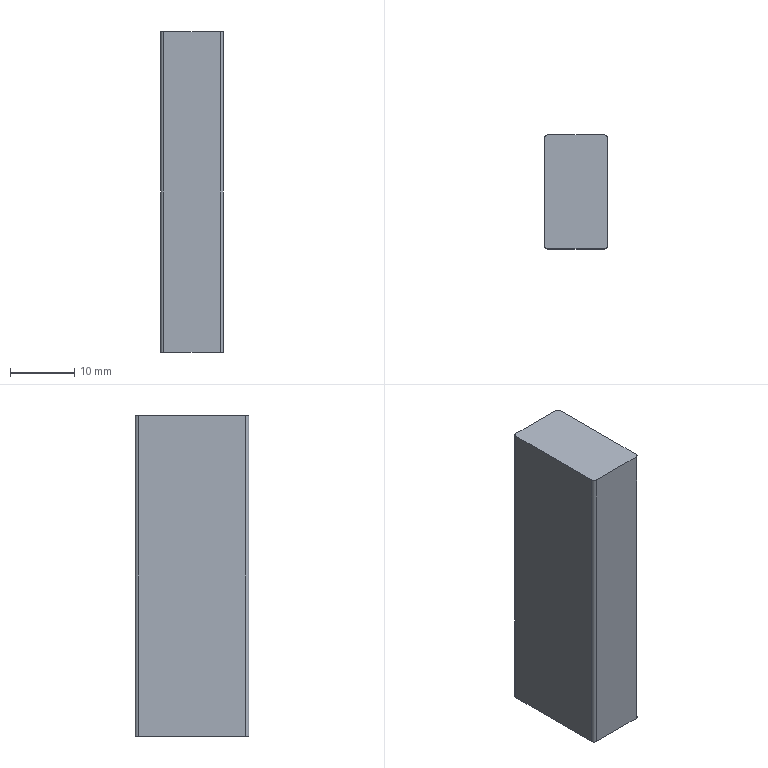Part | NX | features BREP 1 | 1 solid | 10 faces | box 9.8 x 17.754 x 50 mm | volume 8689 mm3 | plane 6 | cylinder 4 | commonest cylinder face diameters 1 x4
STEP:
#1=CARTESIAN_POINT('',(-4.4,8.877,-40.6));
#2=VERTEX_POINT('',#1);
#3=CARTESIAN_POINT('',(-4.9,8.377,-40.6));
#4=VERTEX_POINT('',#3);
#5=CARTESIAN_POINT('',(-4.4,8.377,-40.6));
#6=DIRECTION('',(0.,0.,1.));
#7=DIRECTION('',(1.,0.,0.));
#8=AXIS2_PLACEMENT_3D('',#5,#6,#7);
#9=CIRCLE('',#8,0.5);
#10=EDGE_CURVE('',#2,#4,#9,.T.);
#11=ORIENTED_EDGE('',*,*,#10,.F.);
#12=CARTESIAN_POINT('',(-4.4,8.877,-90.6));
#13=VERTEX_POINT('',#12);
#14=CARTESIAN_POINT('',(-4.4,8.877,-90.6));
#15=DIRECTION('',(0.,0.,1.));
#16=VECTOR('',#15,1000.);
#17=LINE('',#14,#16);
#18=EDGE_CURVE('',#13,#2,#17,.T.);
#19=ORIENTED_EDGE('',*,*,#18,.F.);
#20=CARTESIAN_POINT('',(-4.9,8.377,-90.6));
#21=VERTEX_POINT('',#20);
#22=CARTESIAN_POINT('',(-4.4,8.377,-90.6));
#23=DIRECTION('',(0.,0.,1.));
#24=DIRECTION('',(1.,0.,0.));
#25=AXIS2_PLACEMENT_3D('',#22,#23,#24);
#26=CIRCLE('',#25,0.5);
#27=EDGE_CURVE('',#13,#21,#26,.T.);
#28=ORIENTED_EDGE('',*,*,#27,.T.);
#29=CARTESIAN_POINT('',(-4.9,8.377,-90.6));
#30=DIRECTION('',(0.,0.,1.));
#31=VECTOR('',#30,1000.);
#32=LINE('',#29,#31);
#33=EDGE_CURVE('',#21,#4,#32,.T.);
#34=ORIENTED_EDGE('',*,*,#33,.T.);
#35=EDGE_LOOP('',(#11,#19,#28,#34));
#36=FACE_BOUND('',#35,.T.);
#37=CARTESIAN_POINT('',(-4.4,8.377,-90.6));
#38=DIRECTION('',(0.,0.,1.));
#39=DIRECTION('',(-1.,0.,0.));
#40=AXIS2_PLACEMENT_3D('',#37,#38,#39);
#41=CYLINDRICAL_SURFACE('',#40,0.5);
#42=ADVANCED_FACE('',(#36),#41,.T.);
#43=CARTESIAN_POINT('',(-4.9,-8.377,-40.6));
#44=VERTEX_POINT('',#43);
#45=CARTESIAN_POINT('',(-4.9,-8.377,-40.6));
#46=DIRECTION('',(0.,1.,0.));
#47=VECTOR('',#46,1000.);
#48=LINE('',#45,#47);
#49=EDGE_CURVE('',#44,#4,#48,.T.);
#50=ORIENTED_EDGE('',*,*,#49,.T.);
#51=ORIENTED_EDGE('',*,*,#33,.F.);
#52=CARTESIAN_POINT('',(-4.9,-8.377,-90.6));
#53=VERTEX_POINT('',#52);
#54=CARTESIAN_POINT('',(-4.9,-8.377,-90.6));
#55=DIRECTION('',(0.,1.,0.));
#56=VECTOR('',#55,1000.);
#57=LINE('',#54,#56);
#58=EDGE_CURVE('',#53,#21,#57,.T.);
#59=ORIENTED_EDGE('',*,*,#58,.F.);
#60=CARTESIAN_POINT('',(-4.9,-8.377,-90.6));
#61=DIRECTION('',(0.,0.,1.));
#62=VECTOR('',#61,1000.);
#63=LINE('',#60,#62);
#64=EDGE_CURVE('',#53,#44,#63,.T.);
#65=ORIENTED_EDGE('',*,*,#64,.T.);
#66=EDGE_LOOP('',(#50,#51,#59,#65));
#67=FACE_BOUND('',#66,.T.);
#68=CARTESIAN_POINT('',(-4.9,-8.377,-90.6));
#69=DIRECTION('',(1.,0.,0.));
#70=DIRECTION('',(0.,-1.,0.));
#71=AXIS2_PLACEMENT_3D('',#68,#69,#70);
#72=PLANE('',#71);
#73=ADVANCED_FACE('',(#67),#72,.F.);
#74=CARTESIAN_POINT('',(-4.4,-8.877,-40.6));
#75=VERTEX_POINT('',#74);
#76=CARTESIAN_POINT('',(-4.4,-8.377,-40.6));
#77=DIRECTION('',(0.,0.,1.));
#78=DIRECTION('',(1.,0.,0.));
#79=AXIS2_PLACEMENT_3D('',#76,#77,#78);
#80=CIRCLE('',#79,0.5);
#81=EDGE_CURVE('',#44,#75,#80,.T.);
#82=ORIENTED_EDGE('',*,*,#81,.F.);
#83=ORIENTED_EDGE('',*,*,#64,.F.);
#84=CARTESIAN_POINT('',(-4.4,-8.877,-90.6));
#85=VERTEX_POINT('',#84);
#86=CARTESIAN_POINT('',(-4.4,-8.377,-90.6));
#87=DIRECTION('',(0.,0.,1.));
#88=DIRECTION('',(1.,0.,0.));
#89=AXIS2_PLACEMENT_3D('',#86,#87,#88);
#90=CIRCLE('',#89,0.5);
#91=EDGE_CURVE('',#53,#85,#90,.T.);
#92=ORIENTED_EDGE('',*,*,#91,.T.);
#93=CARTESIAN_POINT('',(-4.4,-8.877,-90.6));
#94=DIRECTION('',(0.,0.,1.));
#95=VECTOR('',#94,1000.);
#96=LINE('',#93,#95);
#97=EDGE_CURVE('',#85,#75,#96,.T.);
#98=ORIENTED_EDGE('',*,*,#97,.T.);
#99=EDGE_LOOP('',(#82,#83,#92,#98));
#100=FACE_BOUND('',#99,.T.);
#101=CARTESIAN_POINT('',(-4.4,-8.377,-90.6));
#102=DIRECTION('',(0.,0.,1.));
#103=DIRECTION('',(-1.,0.,0.));
#104=AXIS2_PLACEMENT_3D('',#101,#102,#103);
#105=CYLINDRICAL_SURFACE('',#104,0.5);
#106=ADVANCED_FACE('',(#100),#105,.T.);
#107=CARTESIAN_POINT('',(4.4,-8.877,-40.6));
#108=VERTEX_POINT('',#107);
#109=CARTESIAN_POINT('',(4.4,-8.877,-40.6));
#110=DIRECTION('',(-1.,0.,0.));
#111=VECTOR('',#110,1000.);
#112=LINE('',#109,#111);
#113=EDGE_CURVE('',#108,#75,#112,.T.);
#114=ORIENTED_EDGE('',*,*,#113,.T.);
#115=ORIENTED_EDGE('',*,*,#97,.F.);
#116=CARTESIAN_POINT('',(4.4,-8.877,-90.6));
#117=VERTEX_POINT('',#116);
#118=CARTESIAN_POINT('',(4.4,-8.877,-90.6));
#119=DIRECTION('',(-1.,0.,0.));
#120=VECTOR('',#119,1000.);
#121=LINE('',#118,#120);
#122=EDGE_CURVE('',#117,#85,#121,.T.);
#123=ORIENTED_EDGE('',*,*,#122,.F.);
#124=CARTESIAN_POINT('',(4.4,-8.877,-90.6));
#125=DIRECTION('',(0.,0.,1.));
#126=VECTOR('',#125,1000.);
#127=LINE('',#124,#126);
#128=EDGE_CURVE('',#117,#108,#127,.T.);
#129=ORIENTED_EDGE('',*,*,#128,.T.);
#130=EDGE_LOOP('',(#114,#115,#123,#129));
#131=FACE_BOUND('',#130,.T.);
#132=CARTESIAN_POINT('',(4.4,-8.877,-90.6));
#133=DIRECTION('',(0.,1.,0.));
#134=DIRECTION('',(0.,0.,-1.));
#135=AXIS2_PLACEMENT_3D('',#132,#133,#134);
#136=PLANE('',#135);
#137=ADVANCED_FACE('',(#131),#136,.F.);
#138=CARTESIAN_POINT('',(4.9,-8.377,-40.6));
#139=VERTEX_POINT('',#138);
#140=CARTESIAN_POINT('',(4.4,-8.377,-40.6));
#141=DIRECTION('',(0.,0.,1.));
#142=DIRECTION('',(1.,0.,0.));
#143=AXIS2_PLACEMENT_3D('',#140,#141,#142);
#144=CIRCLE('',#143,0.5);
#145=EDGE_CURVE('',#108,#139,#144,.T.);
#146=ORIENTED_EDGE('',*,*,#145,.F.);
#147=ORIENTED_EDGE('',*,*,#128,.F.);
#148=CARTESIAN_POINT('',(4.9,-8.377,-90.6));
#149=VERTEX_POINT('',#148);
#150=CARTESIAN_POINT('',(4.4,-8.377,-90.6));
#151=DIRECTION('',(0.,0.,1.));
#152=DIRECTION('',(1.,0.,0.));
#153=AXIS2_PLACEMENT_3D('',#150,#151,#152);
#154=CIRCLE('',#153,0.5);
#155=EDGE_CURVE('',#117,#149,#154,.T.);
#156=ORIENTED_EDGE('',*,*,#155,.T.);
#157=CARTESIAN_POINT('',(4.9,-8.377,-90.6));
#158=DIRECTION('',(0.,0.,1.));
#159=VECTOR('',#158,1000.);
#160=LINE('',#157,#159);
#161=EDGE_CURVE('',#149,#139,#160,.T.);
#162=ORIENTED_EDGE('',*,*,#161,.T.);
#163=EDGE_LOOP('',(#146,#147,#156,#162));
#164=FACE_BOUND('',#163,.T.);
#165=CARTESIAN_POINT('',(4.4,-8.377,-90.6));
#166=DIRECTION('',(0.,0.,1.));
#167=DIRECTION('',(-1.,0.,0.));
#168=AXIS2_PLACEMENT_3D('',#165,#166,#167);
#169=CYLINDRICAL_SURFACE('',#168,0.5);
#170=ADVANCED_FACE('',(#164),#169,.T.);
#171=CARTESIAN_POINT('',(4.9,8.377,-40.6));
#172=VERTEX_POINT('',#171);
#173=CARTESIAN_POINT('',(4.9,8.377,-40.6));
#174=DIRECTION('',(0.,-1.,0.));
#175=VECTOR('',#174,1000.);
#176=LINE('',#173,#175);
#177=EDGE_CURVE('',#172,#139,#176,.T.);
#178=ORIENTED_EDGE('',*,*,#177,.T.);
#179=ORIENTED_EDGE('',*,*,#161,.F.);
#180=CARTESIAN_POINT('',(4.9,8.377,-90.6));
#181=VERTEX_POINT('',#180);
#182=CARTESIAN_POINT('',(4.9,8.377,-90.6));
#183=DIRECTION('',(0.,-1.,0.));
#184=VECTOR('',#183,1000.);
#185=LINE('',#182,#184);
#186=EDGE_CURVE('',#181,#149,#185,.T.);
#187=ORIENTED_EDGE('',*,*,#186,.F.);
#188=CARTESIAN_POINT('',(4.9,8.377,-90.6));
#189=DIRECTION('',(0.,0.,1.));
#190=VECTOR('',#189,1000.);
#191=LINE('',#188,#190);
#192=EDGE_CURVE('',#181,#172,#191,.T.);
#193=ORIENTED_EDGE('',*,*,#192,.T.);
#194=EDGE_LOOP('',(#178,#179,#187,#193));
#195=FACE_BOUND('',#194,.T.);
#196=CARTESIAN_POINT('',(4.9,8.377,-90.6));
#197=DIRECTION('',(-1.,0.,0.));
#198=DIRECTION('',(0.,0.,-1.));
#199=AXIS2_PLACEMENT_3D('',#196,#197,#198);
#200=PLANE('',#199);
#201=ADVANCED_FACE('',(#195),#200,.F.);
#202=CARTESIAN_POINT('',(4.4,8.877,-40.6));
#203=VERTEX_POINT('',#202);
#204=CARTESIAN_POINT('',(4.4,8.377,-40.6));
#205=DIRECTION('',(0.,0.,1.));
#206=DIRECTION('',(1.,0.,0.));
#207=AXIS2_PLACEMENT_3D('',#204,#205,#206);
#208=CIRCLE('',#207,0.5);
#209=EDGE_CURVE('',#172,#203,#208,.T.);
#210=ORIENTED_EDGE('',*,*,#209,.F.);
#211=ORIENTED_EDGE('',*,*,#192,.F.);
#212=CARTESIAN_POINT('',(4.4,8.877,-90.6));
#213=VERTEX_POINT('',#212);
#214=CARTESIAN_POINT('',(4.4,8.377,-90.6));
#215=DIRECTION('',(0.,0.,1.));
#216=DIRECTION('',(1.,0.,0.));
#217=AXIS2_PLACEMENT_3D('',#214,#215,#216);
#218=CIRCLE('',#217,0.5);
#219=EDGE_CURVE('',#181,#213,#218,.T.);
#220=ORIENTED_EDGE('',*,*,#219,.T.);
#221=CARTESIAN_POINT('',(4.4,8.877,-90.6));
#222=DIRECTION('',(0.,0.,1.));
#223=VECTOR('',#222,1000.);
#224=LINE('',#221,#223);
#225=EDGE_CURVE('',#213,#203,#224,.T.);
#226=ORIENTED_EDGE('',*,*,#225,.T.);
#227=EDGE_LOOP('',(#210,#211,#220,#226));
#228=FACE_BOUND('',#227,.T.);
#229=CARTESIAN_POINT('',(4.4,8.377,-90.6));
#230=DIRECTION('',(0.,0.,1.));
#231=DIRECTION('',(-1.,0.,0.));
#232=AXIS2_PLACEMENT_3D('',#229,#230,#231);
#233=CYLINDRICAL_SURFACE('',#232,0.5);
#234=ADVANCED_FACE('',(#228),#233,.T.);
#235=CARTESIAN_POINT('',(-4.4,8.877,-40.6));
#236=DIRECTION('',(1.,0.,0.));
#237=VECTOR('',#236,1000.);
#238=LINE('',#235,#237);
#239=EDGE_CURVE('',#2,#203,#238,.T.);
#240=ORIENTED_EDGE('',*,*,#239,.T.);
#241=ORIENTED_EDGE('',*,*,#225,.F.);
#242=CARTESIAN_POINT('',(-4.4,8.877,-90.6));
#243=DIRECTION('',(1.,0.,0.));
#244=VECTOR('',#243,1000.);
#245=LINE('',#242,#244);
#246=EDGE_CURVE('',#13,#213,#245,.T.);
#247=ORIENTED_EDGE('',*,*,#246,.F.);
#248=ORIENTED_EDGE('',*,*,#18,.T.);
#249=EDGE_LOOP('',(#240,#241,#247,#248));
#250=FACE_BOUND('',#249,.T.);
#251=CARTESIAN_POINT('',(-4.4,8.877,-90.6));
#252=DIRECTION('',(0.,-1.,0.));
#253=DIRECTION('',(-1.,0.,0.));
#254=AXIS2_PLACEMENT_3D('',#251,#252,#253);
#255=PLANE('',#254);
#256=ADVANCED_FACE('',(#250),#255,.F.);
#257=ORIENTED_EDGE('',*,*,#27,.F.);
#258=ORIENTED_EDGE('',*,*,#246,.T.);
#259=ORIENTED_EDGE('',*,*,#219,.F.);
#260=ORIENTED_EDGE('',*,*,#186,.T.);
#261=ORIENTED_EDGE('',*,*,#155,.F.);
#262=ORIENTED_EDGE('',*,*,#122,.T.);
#263=ORIENTED_EDGE('',*,*,#91,.F.);
#264=ORIENTED_EDGE('',*,*,#58,.T.);
#265=EDGE_LOOP('',(#257,#258,#259,#260,#261,#262,#263,#264));
#266=FACE_BOUND('',#265,.T.);
#267=CARTESIAN_POINT('',(-4.4,8.377,-90.6));
#268=DIRECTION('',(0.,0.,1.));
#269=DIRECTION('',(-1.,0.,0.));
#270=AXIS2_PLACEMENT_3D('',#267,#268,#269);
#271=PLANE('',#270);
#272=ADVANCED_FACE('',(#266),#271,.F.);
#273=ORIENTED_EDGE('',*,*,#10,.T.);
#274=ORIENTED_EDGE('',*,*,#49,.F.);
#275=ORIENTED_EDGE('',*,*,#81,.T.);
#276=ORIENTED_EDGE('',*,*,#113,.F.);
#277=ORIENTED_EDGE('',*,*,#145,.T.);
#278=ORIENTED_EDGE('',*,*,#177,.F.);
#279=ORIENTED_EDGE('',*,*,#209,.T.);
#280=ORIENTED_EDGE('',*,*,#239,.F.);
#281=EDGE_LOOP('',(#273,#274,#275,#276,#277,#278,#279,#280));
#282=FACE_BOUND('',#281,.T.);
#283=CARTESIAN_POINT('',(-4.4,8.377,-40.6));
#284=DIRECTION('',(0.,0.,1.));
#285=DIRECTION('',(-1.,0.,0.));
#286=AXIS2_PLACEMENT_3D('',#283,#284,#285);
#287=PLANE('',#286);
#288=ADVANCED_FACE('',(#282),#287,.T.);
#289=CLOSED_SHELL('',(#42,#73,#106,#137,#170,#201,#234,#256,#272,#288));
#290=MANIFOLD_SOLID_BREP('',#289);
#291=(LENGTH_UNIT()NAMED_UNIT(*)SI_UNIT(.MILLI.,.METRE.));
#292=UNCERTAINTY_MEASURE_WITH_UNIT(LENGTH_MEASURE(0.00001),#291,'','');
#293=(NAMED_UNIT(*)PLANE_ANGLE_UNIT()SI_UNIT($,.RADIAN.));
#294=(NAMED_UNIT(*)SI_UNIT($,.STERADIAN.)SOLID_ANGLE_UNIT());
#295=(GEOMETRIC_REPRESENTATION_CONTEXT(3)GLOBAL_UNCERTAINTY_ASSIGNED_CONTEXT((#292))GLOBAL_UNIT_ASSIGNED_CONTEXT((#291,#293,#294))REPRESENTATION_CONTEXT('',''));
#296=ADVANCED_BREP_SHAPE_REPRESENTATION('',(#290),#295);